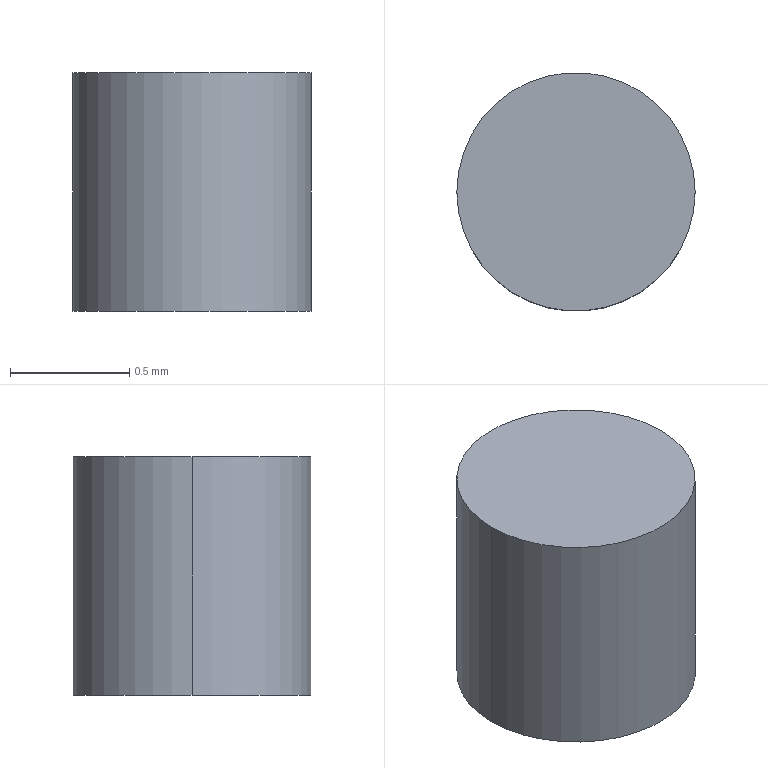Part | SolidWorks | features BaseBody 1 | 1 solid | 4 faces | box 1 x 1 x 1 mm | volume 0.7854 mm3 | cylinder 2 | plane 2 | commonest cylinder face diameters 1 x2
STEP:
#1=CARTESIAN_POINT('',(565.72,76.38,59.053));
#2=VERTEX_POINT('',#1);
#3=CARTESIAN_POINT('',(566.72,76.38,59.053));
#4=VERTEX_POINT('',#3);
#5=CARTESIAN_POINT('',(566.22,76.38,59.053));
#6=DIRECTION('',(0.,0.,-1.));
#7=DIRECTION('',(-1.,0.,0.));
#8=AXIS2_PLACEMENT_3D('',#5,#6,#7);
#9=CIRCLE('',#8,0.5);
#10=EDGE_CURVE('',#2,#4,#9,.T.);
#11=ORIENTED_EDGE('',*,*,#10,.T.);
#12=CARTESIAN_POINT('',(566.72,76.38,58.053));
#13=VERTEX_POINT('',#12);
#14=CARTESIAN_POINT('',(566.72,76.38,59.053));
#15=DIRECTION('',(0.,0.,-1.));
#16=VECTOR('',#15,1000.);
#17=LINE('',#14,#16);
#18=EDGE_CURVE('',#4,#13,#17,.T.);
#19=ORIENTED_EDGE('',*,*,#18,.T.);
#20=CARTESIAN_POINT('',(565.72,76.38,58.053));
#21=VERTEX_POINT('',#20);
#22=CARTESIAN_POINT('',(566.22,76.38,58.053));
#23=DIRECTION('',(0.,0.,1.));
#24=DIRECTION('',(-1.,0.,0.));
#25=AXIS2_PLACEMENT_3D('',#22,#23,#24);
#26=CIRCLE('',#25,0.5);
#27=EDGE_CURVE('',#13,#21,#26,.T.);
#28=ORIENTED_EDGE('',*,*,#27,.T.);
#29=CARTESIAN_POINT('',(565.72,76.38,59.053));
#30=DIRECTION('',(0.,0.,-1.));
#31=VECTOR('',#30,1000.);
#32=LINE('',#29,#31);
#33=EDGE_CURVE('',#2,#21,#32,.T.);
#34=ORIENTED_EDGE('',*,*,#33,.F.);
#35=EDGE_LOOP('',(#11,#19,#28,#34));
#36=FACE_OUTER_BOUND('',#35,.T.);
#37=CARTESIAN_POINT('',(566.22,76.38,59.053));
#38=DIRECTION('',(0.,0.,-1.));
#39=DIRECTION('',(-1.,0.,0.));
#40=AXIS2_PLACEMENT_3D('',#37,#38,#39);
#41=CYLINDRICAL_SURFACE('',#40,0.5);
#42=ADVANCED_FACE('',(#36),#41,.T.);
#43=ORIENTED_EDGE('',*,*,#18,.F.);
#44=CARTESIAN_POINT('',(566.22,76.38,59.053));
#45=DIRECTION('',(0.,0.,-1.));
#46=DIRECTION('',(-1.,0.,0.));
#47=AXIS2_PLACEMENT_3D('',#44,#45,#46);
#48=CIRCLE('',#47,0.5);
#49=EDGE_CURVE('',#4,#2,#48,.T.);
#50=ORIENTED_EDGE('',*,*,#49,.T.);
#51=ORIENTED_EDGE('',*,*,#33,.T.);
#52=CARTESIAN_POINT('',(566.22,76.38,58.053));
#53=DIRECTION('',(0.,0.,1.));
#54=DIRECTION('',(-1.,0.,0.));
#55=AXIS2_PLACEMENT_3D('',#52,#53,#54);
#56=CIRCLE('',#55,0.5);
#57=EDGE_CURVE('',#21,#13,#56,.T.);
#58=ORIENTED_EDGE('',*,*,#57,.T.);
#59=EDGE_LOOP('',(#43,#50,#51,#58));
#60=FACE_OUTER_BOUND('',#59,.T.);
#61=CARTESIAN_POINT('',(566.22,76.38,59.053));
#62=DIRECTION('',(0.,0.,-1.));
#63=DIRECTION('',(-1.,0.,0.));
#64=AXIS2_PLACEMENT_3D('',#61,#62,#63);
#65=CYLINDRICAL_SURFACE('',#64,0.5);
#66=ADVANCED_FACE('',(#60),#65,.T.);
#67=ORIENTED_EDGE('',*,*,#57,.F.);
#68=ORIENTED_EDGE('',*,*,#27,.F.);
#69=EDGE_LOOP('',(#67,#68));
#70=FACE_OUTER_BOUND('',#69,.T.);
#71=CARTESIAN_POINT('',(566.265,76.38,58.053));
#72=DIRECTION('',(0.,0.,-1.));
#73=DIRECTION('',(-1.,0.,0.));
#74=AXIS2_PLACEMENT_3D('',#71,#72,#73);
#75=PLANE('',#74);
#76=ADVANCED_FACE('',(#70),#75,.T.);
#77=ORIENTED_EDGE('',*,*,#10,.F.);
#78=ORIENTED_EDGE('',*,*,#49,.F.);
#79=EDGE_LOOP('',(#77,#78));
#80=FACE_OUTER_BOUND('',#79,.T.);
#81=CARTESIAN_POINT('',(566.265,76.38,59.053));
#82=DIRECTION('',(0.,0.,1.));
#83=DIRECTION('',(1.,0.,0.));
#84=AXIS2_PLACEMENT_3D('',#81,#82,#83);
#85=PLANE('',#84);
#86=ADVANCED_FACE('',(#80),#85,.T.);
#87=CLOSED_SHELL('',(#42,#66,#76,#86));
#88=MANIFOLD_SOLID_BREP('',#87);
#89=CARTESIAN_POINT('',(0.,0.,0.));
#90=DIRECTION('',(0.,0.,1.));
#91=DIRECTION('',(1.,0.,0.));
#92=AXIS2_PLACEMENT_3D('',#89,#90,#91);
#93=(LENGTH_UNIT()NAMED_UNIT(*)SI_UNIT(.MILLI.,.METRE.));
#94=UNCERTAINTY_MEASURE_WITH_UNIT(LENGTH_MEASURE(0.00001),#93,'','');
#95=(NAMED_UNIT(*)PLANE_ANGLE_UNIT()SI_UNIT($,.RADIAN.));
#96=(NAMED_UNIT(*)SI_UNIT($,.STERADIAN.)SOLID_ANGLE_UNIT());
#97=(GEOMETRIC_REPRESENTATION_CONTEXT(3)GLOBAL_UNCERTAINTY_ASSIGNED_CONTEXT((#94))GLOBAL_UNIT_ASSIGNED_CONTEXT((#93,#95,#96))REPRESENTATION_CONTEXT('',''));
#98=ADVANCED_BREP_SHAPE_REPRESENTATION('',(#88,#92),#97);